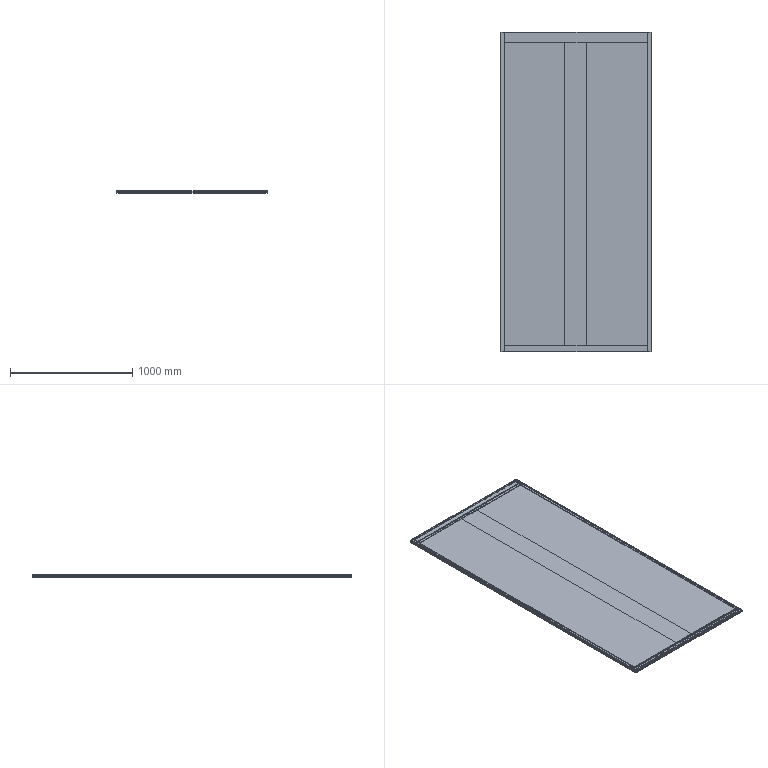Part | 5 solids | 338 faces | box 1230 x 2616 x 20.2 mm | volume 31993862 mm3 | cylinder 180 | plane 158 | commonest cylinder face diameters 0.6 x48 13 x48 0.4 x27 1 x21 9 x16 7.2 x12